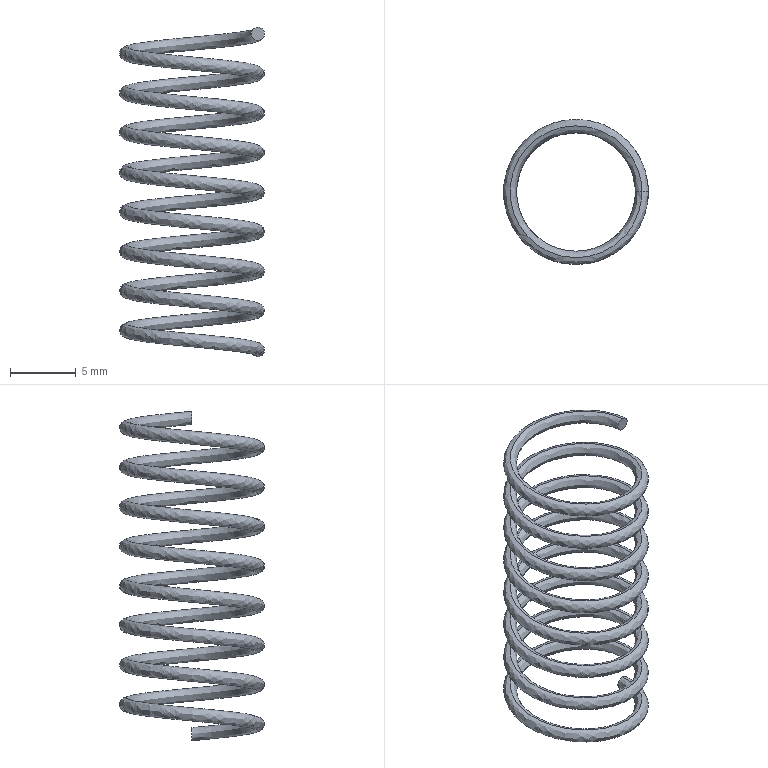Part | SolidWorks | features Helix 1, RefAxis 1, Sweep 1 | 1 solid | 4 faces | box 11 x 11 x 25 mm | volume 196.371 mm3 | spline 2 | plane 2